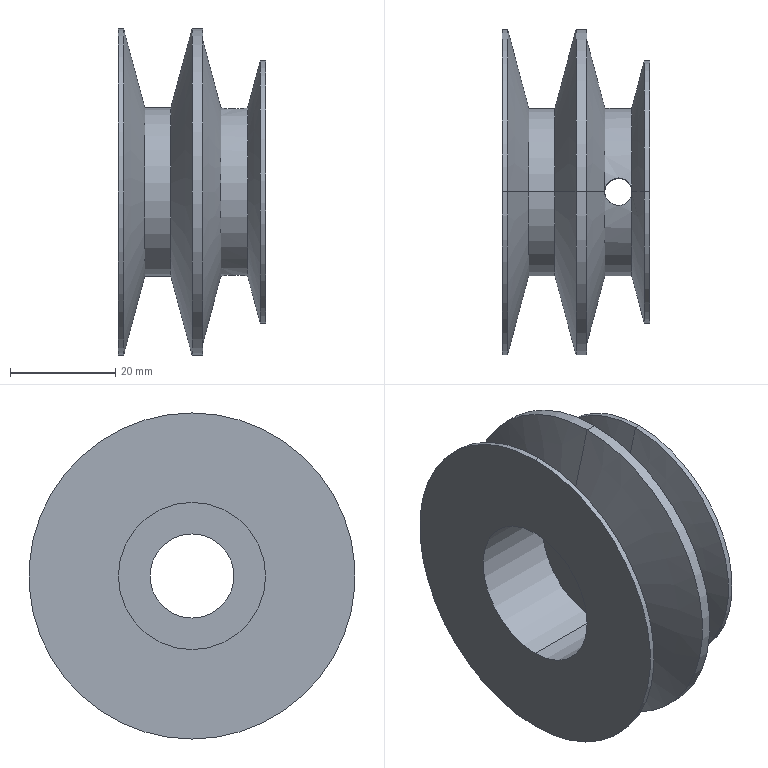Part | SolidWorks | features ICE 2, 3DProfileFeature 1, HoleWzd 1, Revolution 1 | 1 solid | 32 faces | box 28 x 62 x 62 mm | volume 29856 mm3 | cylinder 18 | cone 8 | plane 6 | commonest cylinder face diameters 5.22 x4 32 x4 62 x4 16 x2 28 x2 50 x2
STEP:
#1=CARTESIAN_POINT('',(-21.548,2.63,7.555));
#2=VERTEX_POINT('',#1);
#3=CARTESIAN_POINT('',(-24.158,0.,8.));
#4=VERTEX_POINT('',#3);
#5=CARTESIAN_POINT('',(-21.548,2.63,7.555));
#6=CARTESIAN_POINT('',(-21.72,2.63,7.555));
#7=CARTESIAN_POINT('',(-21.893,2.613,7.561));
#8=CARTESIAN_POINT('',(-22.233,2.545,7.585));
#9=CARTESIAN_POINT('',(-22.397,2.494,7.602));
#10=CARTESIAN_POINT('',(-22.713,2.362,7.644));
#11=CARTESIAN_POINT('',(-22.866,2.279,7.669));
#12=CARTESIAN_POINT('',(-23.149,2.089,7.723));
#13=CARTESIAN_POINT('',(-23.28,1.981,7.752));
#14=CARTESIAN_POINT('',(-23.642,1.616,7.839));
#15=CARTESIAN_POINT('',(-23.833,1.329,7.895));
#16=CARTESIAN_POINT('',(-24.029,0.8493,7.956));
#17=CARTESIAN_POINT('',(-24.078,0.6851,7.972));
#18=CARTESIAN_POINT('',(-24.143,0.3479,7.994));
#19=CARTESIAN_POINT('',(-24.159,0.1727,8.));
#20=CARTESIAN_POINT('',(-24.158,0.,8.));
#21=B_SPLINE_CURVE_WITH_KNOTS('',3,(#5,#6,#7,#8,#9,#10,#11,#12,#13,#14,#15,#16,#17,#18,#19,#20),.UNSPECIFIED.,.F.,.F.,(4,2,2,2,2,2,2,4),(0.008216,0.008732,0.009248,0.009764,0.01028,0.01131,0.01183,0.01234),.UNSPECIFIED.);
#22=EDGE_CURVE('',#2,#4,#21,.T.);
#23=ORIENTED_EDGE('',*,*,#22,.F.);
#24=CARTESIAN_POINT('',(-21.548,2.652,15.779));
#25=VERTEX_POINT('',#24);
#26=CARTESIAN_POINT('',(-21.548,2.653,15.993));
#27=DIRECTION('',(0.,0.002678,1.));
#28=VECTOR('',#27,1000.);
#29=LINE('',#26,#28);
#30=EDGE_CURVE('',#2,#25,#29,.T.);
#31=ORIENTED_EDGE('',*,*,#30,.T.);
#32=CARTESIAN_POINT('',(-24.127,0.4433,15.994));
#33=VERTEX_POINT('',#32);
#34=CARTESIAN_POINT('',(-24.127,0.4433,15.994));
#35=CARTESIAN_POINT('',(-24.079,0.7512,15.985));
#36=CARTESIAN_POINT('',(-23.979,1.043,15.968));
#37=CARTESIAN_POINT('',(-23.752,1.449,15.935));
#38=CARTESIAN_POINT('',(-23.666,1.576,15.923));
#39=CARTESIAN_POINT('',(-23.472,1.813,15.897));
#40=CARTESIAN_POINT('',(-23.363,1.924,15.884));
#41=CARTESIAN_POINT('',(-23.129,2.125,15.859));
#42=CARTESIAN_POINT('',(-23.004,2.214,15.846));
#43=CARTESIAN_POINT('',(-22.74,2.369,15.824));
#44=CARTESIAN_POINT('',(-22.599,2.436,15.814));
#45=CARTESIAN_POINT('',(-22.309,2.543,15.797));
#46=CARTESIAN_POINT('',(-22.161,2.584,15.79));
#47=CARTESIAN_POINT('',(-21.859,2.638,15.781));
#48=CARTESIAN_POINT('',(-21.702,2.652,15.779));
#49=CARTESIAN_POINT('',(-21.548,2.652,15.779));
#50=B_SPLINE_CURVE_WITH_KNOTS('',3,(#34,#35,#36,#37,#38,#39,#40,#41,#42,#43,#44,#45,#46,#47,#48,#49),.UNSPECIFIED.,.F.,.F.,(4,2,2,2,2,2,2,4),(0.,0.0009215,0.001382,0.001843,0.002304,0.002764,0.003225,0.003686),.UNSPECIFIED.);
#51=EDGE_CURVE('',#33,#25,#50,.T.);
#52=ORIENTED_EDGE('',*,*,#51,.F.);
#53=CARTESIAN_POINT('',(-24.128,0.435,15.999));
#54=VERTEX_POINT('',#53);
#55=CARTESIAN_POINT('',(-24.128,0.435,15.999));
#56=CARTESIAN_POINT('',(-24.128,0.4378,15.997));
#57=CARTESIAN_POINT('',(-24.127,0.4406,15.996));
#58=CARTESIAN_POINT('',(-24.127,0.4433,15.994));
#59=B_SPLINE_CURVE_WITH_KNOTS('',3,(#55,#56,#57,#58),.UNSPECIFIED.,.F.,.F.,(4,4),(0.0008614,0.0008711),.UNSPECIFIED.);
#60=EDGE_CURVE('',#54,#33,#59,.T.);
#61=ORIENTED_EDGE('',*,*,#60,.F.);
#62=CARTESIAN_POINT('',(-24.128,-0.3493,16.001));
#63=VERTEX_POINT('',#62);
#64=CARTESIAN_POINT('',(-21.548,0.04285,16.));
#65=DIRECTION('',(0.,0.002678,1.));
#66=DIRECTION('',(0.,-1.,0.002678));
#67=AXIS2_PLACEMENT_3D('',#64,#65,#66);
#68=CIRCLE('',#67,2.61);
#69=EDGE_CURVE('',#54,#63,#68,.T.);
#70=ORIENTED_EDGE('',*,*,#69,.T.);
#71=CARTESIAN_POINT('',(-24.127,-0.3577,15.996));
#72=VERTEX_POINT('',#71);
#73=CARTESIAN_POINT('',(-24.127,-0.3577,15.996));
#74=CARTESIAN_POINT('',(-24.127,-0.3549,15.998));
#75=CARTESIAN_POINT('',(-24.128,-0.3521,15.999));
#76=CARTESIAN_POINT('',(-24.128,-0.3493,16.001));
#77=B_SPLINE_CURVE_WITH_KNOTS('',3,(#73,#74,#75,#76),.UNSPECIFIED.,.F.,.F.,(4,4),(0.00002434,0.00003413),.UNSPECIFIED.);
#78=EDGE_CURVE('',#72,#63,#77,.T.);
#79=ORIENTED_EDGE('',*,*,#78,.F.);
#80=CARTESIAN_POINT('',(-21.548,-2.568,15.793));
#81=VERTEX_POINT('',#80);
#82=CARTESIAN_POINT('',(-21.548,-2.568,15.793));
#83=CARTESIAN_POINT('',(-21.703,-2.568,15.793));
#84=CARTESIAN_POINT('',(-21.858,-2.554,15.795));
#85=CARTESIAN_POINT('',(-22.16,-2.499,15.804));
#86=CARTESIAN_POINT('',(-22.309,-2.459,15.81));
#87=CARTESIAN_POINT('',(-22.746,-2.297,15.835));
#88=CARTESIAN_POINT('',(-23.011,-2.141,15.857));
#89=CARTESIAN_POINT('',(-23.364,-1.838,15.894));
#90=CARTESIAN_POINT('',(-23.471,-1.728,15.907));
#91=CARTESIAN_POINT('',(-23.665,-1.491,15.931));
#92=CARTESIAN_POINT('',(-23.752,-1.363,15.942));
#93=CARTESIAN_POINT('',(-23.978,-0.9574,15.974));
#94=CARTESIAN_POINT('',(-24.079,-0.6654,15.989));
#95=CARTESIAN_POINT('',(-24.127,-0.3577,15.996));
#96=B_SPLINE_CURVE_WITH_KNOTS('',3,(#82,#83,#84,#85,#86,#87,#88,#89,#90,#91,#92,#93,#94,#95),.UNSPECIFIED.,.F.,.F.,(4,2,2,2,2,2,4),(0.003428,0.003888,0.004349,0.00527,0.005731,0.006191,0.007113),.UNSPECIFIED.);
#97=EDGE_CURVE('',#81,#72,#96,.T.);
#98=ORIENTED_EDGE('',*,*,#97,.F.);
#99=CARTESIAN_POINT('',(-21.548,-2.59,7.569));
#100=VERTEX_POINT('',#99);
#101=CARTESIAN_POINT('',(-21.548,-2.567,16.007));
#102=DIRECTION('',(0.,0.002678,1.));
#103=VECTOR('',#102,1000.);
#104=LINE('',#101,#103);
#105=EDGE_CURVE('',#100,#81,#104,.T.);
#106=ORIENTED_EDGE('',*,*,#105,.F.);
#107=CARTESIAN_POINT('',(-24.158,0.,8.));
#108=CARTESIAN_POINT('',(-24.156,-0.1709,8.));
#109=CARTESIAN_POINT('',(-24.138,-0.3402,7.995));
#110=CARTESIAN_POINT('',(-24.069,-0.6754,7.973));
#111=CARTESIAN_POINT('',(-24.017,-0.8402,7.957));
#112=CARTESIAN_POINT('',(-23.819,-1.308,7.899));
#113=CARTESIAN_POINT('',(-23.625,-1.595,7.843));
#114=CARTESIAN_POINT('',(-23.267,-1.951,7.76));
#115=CARTESIAN_POINT('',(-23.134,-2.059,7.731));
#116=CARTESIAN_POINT('',(-22.852,-2.246,7.679));
#117=CARTESIAN_POINT('',(-22.704,-2.326,7.655));
#118=CARTESIAN_POINT('',(-22.39,-2.456,7.614));
#119=CARTESIAN_POINT('',(-22.224,-2.506,7.597));
#120=CARTESIAN_POINT('',(-21.891,-2.573,7.575));
#121=CARTESIAN_POINT('',(-21.721,-2.59,7.569));
#122=CARTESIAN_POINT('',(-21.548,-2.59,7.569));
#123=B_SPLINE_CURVE_WITH_KNOTS('',3,(#107,#108,#109,#110,#111,#112,#113,#114,#115,#116,#117,#118,#119,#120,#121,#122),.UNSPECIFIED.,.F.,.F.,(4,2,2,2,2,2,2,4),(0.01234,0.01285,0.01337,0.01439,0.0149,0.01541,0.01592,0.01643),.UNSPECIFIED.);
#124=EDGE_CURVE('',#4,#100,#123,.T.);
#125=ORIENTED_EDGE('',*,*,#124,.F.);
#126=EDGE_LOOP('',(#23,#31,#52,#61,#70,#79,#98,#106,#125));
#127=FACE_OUTER_BOUND('',#126,.T.);
#128=CARTESIAN_POINT('',(-21.548,0.04285,16.));
#129=DIRECTION('',(0.,0.002678,1.));
#130=DIRECTION('',(0.,-1.,0.002678));
#131=AXIS2_PLACEMENT_3D('',#128,#129,#130);
#132=CYLINDRICAL_SURFACE('',#131,2.61);
#133=ADVANCED_FACE('',(#127),#132,.F.);
#134=CARTESIAN_POINT('',(-21.548,2.568,-15.793));
#135=VERTEX_POINT('',#134);
#136=CARTESIAN_POINT('',(-24.127,0.3577,-15.996));
#137=VERTEX_POINT('',#136);
#138=CARTESIAN_POINT('',(-21.548,2.568,-15.793));
#139=CARTESIAN_POINT('',(-21.703,2.568,-15.793));
#140=CARTESIAN_POINT('',(-21.858,2.554,-15.795));
#141=CARTESIAN_POINT('',(-22.16,2.499,-15.804));
#142=CARTESIAN_POINT('',(-22.309,2.459,-15.81));
#143=CARTESIAN_POINT('',(-22.746,2.297,-15.835));
#144=CARTESIAN_POINT('',(-23.011,2.141,-15.857));
#145=CARTESIAN_POINT('',(-23.364,1.838,-15.894));
#146=CARTESIAN_POINT('',(-23.471,1.728,-15.907));
#147=CARTESIAN_POINT('',(-23.665,1.491,-15.931));
#148=CARTESIAN_POINT('',(-23.752,1.363,-15.942));
#149=CARTESIAN_POINT('',(-23.978,0.9574,-15.974));
#150=CARTESIAN_POINT('',(-24.079,0.6654,-15.989));
#151=CARTESIAN_POINT('',(-24.127,0.3577,-15.996));
#152=B_SPLINE_CURVE_WITH_KNOTS('',3,(#138,#139,#140,#141,#142,#143,#144,#145,#146,#147,#148,#149,#150,#151),.UNSPECIFIED.,.F.,.F.,(4,2,2,2,2,2,4),(0.003428,0.003888,0.004349,0.00527,0.005731,0.006191,0.007113),.UNSPECIFIED.);
#153=EDGE_CURVE('',#135,#137,#152,.T.);
#154=ORIENTED_EDGE('',*,*,#153,.F.);
#155=CARTESIAN_POINT('',(-21.548,2.59,-7.569));
#156=VERTEX_POINT('',#155);
#157=CARTESIAN_POINT('',(-21.548,2.653,15.993));
#158=DIRECTION('',(0.,0.002678,1.));
#159=VECTOR('',#158,1000.);
#160=LINE('',#157,#159);
#161=EDGE_CURVE('',#135,#156,#160,.T.);
#162=ORIENTED_EDGE('',*,*,#161,.T.);
#163=CARTESIAN_POINT('',(-24.158,0.,-8.));
#164=VERTEX_POINT('',#163);
#165=CARTESIAN_POINT('',(-24.158,0.,-8.));
#166=CARTESIAN_POINT('',(-24.156,0.1729,-8.));
#167=CARTESIAN_POINT('',(-24.138,0.3425,-7.994));
#168=CARTESIAN_POINT('',(-24.069,0.6756,-7.973));
#169=CARTESIAN_POINT('',(-24.017,0.8408,-7.957));
#170=CARTESIAN_POINT('',(-23.884,1.154,-7.918));
#171=CARTESIAN_POINT('',(-23.804,1.303,-7.895));
#172=CARTESIAN_POINT('',(-23.614,1.583,-7.843));
#173=CARTESIAN_POINT('',(-23.504,1.715,-7.815));
#174=CARTESIAN_POINT('',(-23.146,2.07,-7.731));
#175=CARTESIAN_POINT('',(-22.857,2.262,-7.675));
#176=CARTESIAN_POINT('',(-22.389,2.456,-7.614));
#177=CARTESIAN_POINT('',(-22.224,2.506,-7.597));
#178=CARTESIAN_POINT('',(-21.888,2.573,-7.575));
#179=CARTESIAN_POINT('',(-21.719,2.59,-7.569));
#180=CARTESIAN_POINT('',(-21.548,2.59,-7.569));
#181=B_SPLINE_CURVE_WITH_KNOTS('',3,(#165,#166,#167,#168,#169,#170,#171,#172,#173,#174,#175,#176,#177,#178,#179,#180),.UNSPECIFIED.,.F.,.F.,(4,2,2,2,2,2,2,4),(0.,0.000511,0.001022,0.001533,0.002044,0.003066,0.003577,0.004088),.UNSPECIFIED.);
#182=EDGE_CURVE('',#164,#156,#181,.T.);
#183=ORIENTED_EDGE('',*,*,#182,.F.);
#184=CARTESIAN_POINT('',(-21.548,-2.63,-7.555));
#185=VERTEX_POINT('',#184);
#186=CARTESIAN_POINT('',(-21.548,-2.63,-7.555));
#187=CARTESIAN_POINT('',(-21.721,-2.63,-7.555));
#188=CARTESIAN_POINT('',(-21.892,-2.613,-7.561));
#189=CARTESIAN_POINT('',(-22.231,-2.545,-7.584));
#190=CARTESIAN_POINT('',(-22.398,-2.494,-7.602));
#191=CARTESIAN_POINT('',(-22.871,-2.296,-7.665));
#192=CARTESIAN_POINT('',(-23.161,-2.1,-7.723));
#193=CARTESIAN_POINT('',(-23.52,-1.739,-7.81));
#194=CARTESIAN_POINT('',(-23.63,-1.604,-7.839));
#195=CARTESIAN_POINT('',(-23.818,-1.32,-7.892));
#196=CARTESIAN_POINT('',(-23.898,-1.169,-7.916));
#197=CARTESIAN_POINT('',(-24.028,-0.8517,-7.956));
#198=CARTESIAN_POINT('',(-24.078,-0.6839,-7.973));
#199=CARTESIAN_POINT('',(-24.143,-0.3463,-7.994));
#200=CARTESIAN_POINT('',(-24.159,-0.1746,-8.));
#201=CARTESIAN_POINT('',(-24.158,0.,-8.));
#202=B_SPLINE_CURVE_WITH_KNOTS('',3,(#186,#187,#188,#189,#190,#191,#192,#193,#194,#195,#196,#197,#198,#199,#200,#201),.UNSPECIFIED.,.F.,.F.,(4,2,2,2,2,2,2,4),(0.0123,0.01282,0.01333,0.01437,0.01488,0.0154,0.01591,0.01643),.UNSPECIFIED.);
#203=EDGE_CURVE('',#185,#164,#202,.T.);
#204=ORIENTED_EDGE('',*,*,#203,.F.);
#205=CARTESIAN_POINT('',(-21.548,-2.652,-15.779));
#206=VERTEX_POINT('',#205);
#207=CARTESIAN_POINT('',(-21.548,-2.567,16.007));
#208=DIRECTION('',(0.,0.002678,1.));
#209=VECTOR('',#208,1000.);
#210=LINE('',#207,#209);
#211=EDGE_CURVE('',#206,#185,#210,.T.);
#212=ORIENTED_EDGE('',*,*,#211,.F.);
#213=CARTESIAN_POINT('',(-24.127,-0.4433,-15.994));
#214=VERTEX_POINT('',#213);
#215=CARTESIAN_POINT('',(-24.127,-0.4433,-15.994));
#216=CARTESIAN_POINT('',(-24.079,-0.7512,-15.985));
#217=CARTESIAN_POINT('',(-23.979,-1.043,-15.968));
#218=CARTESIAN_POINT('',(-23.752,-1.449,-15.935));
#219=CARTESIAN_POINT('',(-23.666,-1.576,-15.923));
#220=CARTESIAN_POINT('',(-23.472,-1.813,-15.897));
#221=CARTESIAN_POINT('',(-23.363,-1.924,-15.884));
#222=CARTESIAN_POINT('',(-23.129,-2.125,-15.859));
#223=CARTESIAN_POINT('',(-23.004,-2.214,-15.846));
#224=CARTESIAN_POINT('',(-22.74,-2.369,-15.824));
#225=CARTESIAN_POINT('',(-22.599,-2.436,-15.814));
#226=CARTESIAN_POINT('',(-22.309,-2.543,-15.797));
#227=CARTESIAN_POINT('',(-22.161,-2.584,-15.79));
#228=CARTESIAN_POINT('',(-21.859,-2.638,-15.781));
#229=CARTESIAN_POINT('',(-21.702,-2.652,-15.779));
#230=CARTESIAN_POINT('',(-21.548,-2.652,-15.779));
#231=B_SPLINE_CURVE_WITH_KNOTS('',3,(#215,#216,#217,#218,#219,#220,#221,#222,#223,#224,#225,#226,#227,#228,#229,#230),.UNSPECIFIED.,.F.,.F.,(4,2,2,2,2,2,2,4),(0.,0.0009215,0.001382,0.001843,0.002304,0.002764,0.003225,0.003686),.UNSPECIFIED.);
#232=EDGE_CURVE('',#214,#206,#231,.T.);
#233=ORIENTED_EDGE('',*,*,#232,.F.);
#234=CARTESIAN_POINT('',(-24.158,0.,-16.114));
#235=VERTEX_POINT('',#234);
#236=CARTESIAN_POINT('',(-24.158,0.,-16.114));
#237=CARTESIAN_POINT('',(-24.159,-0.07704,-16.119));
#238=CARTESIAN_POINT('',(-24.157,-0.1564,-16.11));
#239=CARTESIAN_POINT('',(-24.146,-0.3055,-16.067));
#240=CARTESIAN_POINT('',(-24.137,-0.377,-16.034));
#241=CARTESIAN_POINT('',(-24.127,-0.4433,-15.994));
#242=B_SPLINE_CURVE_WITH_KNOTS('',3,(#236,#237,#238,#239,#240,#241),.UNSPECIFIED.,.F.,.F.,(4,2,4),(0.0004054,0.0006383,0.0008711),.UNSPECIFIED.);
#243=EDGE_CURVE('',#235,#214,#242,.T.);
#244=ORIENTED_EDGE('',*,*,#243,.F.);
#245=CARTESIAN_POINT('',(-24.127,0.3577,-15.996));
#246=CARTESIAN_POINT('',(-24.144,0.249,-16.061));
#247=CARTESIAN_POINT('',(-24.155,0.1261,-16.106));
#248=CARTESIAN_POINT('',(-24.158,0.,-16.114));
#249=B_SPLINE_CURVE_WITH_KNOTS('',3,(#245,#246,#247,#248),.UNSPECIFIED.,.F.,.F.,(4,4),(0.00002434,0.0004054),.UNSPECIFIED.);
#250=EDGE_CURVE('',#137,#235,#249,.T.);
#251=ORIENTED_EDGE('',*,*,#250,.F.);
#252=EDGE_LOOP('',(#154,#162,#183,#204,#212,#233,#244,#251));
#253=FACE_OUTER_BOUND('',#252,.T.);
#254=CARTESIAN_POINT('',(-21.548,0.04285,16.));
#255=DIRECTION('',(0.,0.002678,1.));
#256=DIRECTION('',(0.,-1.,0.002678));
#257=AXIS2_PLACEMENT_3D('',#254,#255,#256);
#258=CYLINDRICAL_SURFACE('',#257,2.61);
#259=ADVANCED_FACE('',(#253),#258,.F.);
#260=CARTESIAN_POINT('',(-27.61,0.,14.));
#261=VERTEX_POINT('',#260);
#262=CARTESIAN_POINT('',(-27.61,0.,-14.));
#263=VERTEX_POINT('',#262);
#264=CARTESIAN_POINT('',(-27.61,0.,0.));
#265=DIRECTION('',(1.,0.,0.));
#266=DIRECTION('',(0.,0.,1.));
#267=AXIS2_PLACEMENT_3D('',#264,#265,#266);
#268=CIRCLE('',#267,14.);
#269=EDGE_CURVE('',#261,#263,#268,.T.);
#270=ORIENTED_EDGE('',*,*,#269,.T.);
#271=CARTESIAN_POINT('',(-43.61,0.,-14.));
#272=VERTEX_POINT('',#271);
#273=CARTESIAN_POINT('',(11.988,0.,-14.));
#274=DIRECTION('',(-1.,0.,0.));
#275=VECTOR('',#274,1000.);
#276=LINE('',#273,#275);
#277=EDGE_CURVE('',#263,#272,#276,.T.);
#278=ORIENTED_EDGE('',*,*,#277,.T.);
#279=CARTESIAN_POINT('',(-43.61,0.,14.));
#280=VERTEX_POINT('',#279);
#281=CARTESIAN_POINT('',(-43.61,0.,0.));
#282=DIRECTION('',(-1.,0.,0.));
#283=DIRECTION('',(0.,0.,1.));
#284=AXIS2_PLACEMENT_3D('',#281,#282,#283);
#285=CIRCLE('',#284,14.);
#286=EDGE_CURVE('',#272,#280,#285,.T.);
#287=ORIENTED_EDGE('',*,*,#286,.T.);
#288=CARTESIAN_POINT('',(11.988,0.,14.));
#289=DIRECTION('',(-1.,0.,0.));
#290=VECTOR('',#289,1000.);
#291=LINE('',#288,#290);
#292=EDGE_CURVE('',#261,#280,#291,.T.);
#293=ORIENTED_EDGE('',*,*,#292,.F.);
#294=EDGE_LOOP('',(#270,#278,#287,#293));
#295=FACE_OUTER_BOUND('',#294,.T.);
#296=CARTESIAN_POINT('',(11.988,0.,0.));
#297=DIRECTION('',(-1.,0.,0.));
#298=DIRECTION('',(0.,0.,1.));
#299=AXIS2_PLACEMENT_3D('',#296,#297,#298);
#300=CYLINDRICAL_SURFACE('',#299,14.);
#301=ADVANCED_FACE('',(#295),#300,.F.);
#302=CARTESIAN_POINT('',(-15.61,0.,25.));
#303=VERTEX_POINT('',#302);
#304=CARTESIAN_POINT('',(-15.61,0.,-25.));
#305=VERTEX_POINT('',#304);
#306=CARTESIAN_POINT('',(-15.61,0.,0.));
#307=DIRECTION('',(-1.,0.,0.));
#308=DIRECTION('',(0.,0.,1.));
#309=AXIS2_PLACEMENT_3D('',#306,#307,#308);
#310=CIRCLE('',#309,25.);
#311=EDGE_CURVE('',#303,#305,#310,.T.);
#312=ORIENTED_EDGE('',*,*,#311,.T.);
#313=CARTESIAN_POINT('',(-16.61,0.,-25.));
#314=VERTEX_POINT('',#313);
#315=CARTESIAN_POINT('',(-65.147,0.,-25.));
#316=DIRECTION('',(-1.,0.,0.));
#317=VECTOR('',#316,1000.);
#318=LINE('',#315,#317);
#319=EDGE_CURVE('',#305,#314,#318,.T.);
#320=ORIENTED_EDGE('',*,*,#319,.T.);
#321=CARTESIAN_POINT('',(-16.61,0.,25.));
#322=VERTEX_POINT('',#321);
#323=CARTESIAN_POINT('',(-16.61,0.,0.));
#324=DIRECTION('',(-1.,0.,0.));
#325=DIRECTION('',(0.,0.,1.));
#326=AXIS2_PLACEMENT_3D('',#323,#324,#325);
#327=CIRCLE('',#326,25.);
#328=EDGE_CURVE('',#322,#314,#327,.T.);
#329=ORIENTED_EDGE('',*,*,#328,.F.);
#330=CARTESIAN_POINT('',(-65.147,0.,25.));
#331=DIRECTION('',(-1.,0.,0.));
#332=VECTOR('',#331,1000.);
#333=LINE('',#330,#332);
#334=EDGE_CURVE('',#303,#322,#333,.T.);
#335=ORIENTED_EDGE('',*,*,#334,.F.);
#336=EDGE_LOOP('',(#312,#320,#329,#335));
#337=FACE_OUTER_BOUND('',#336,.T.);
#338=CARTESIAN_POINT('',(-65.147,0.,0.));
#339=DIRECTION('',(-1.,0.,0.));
#340=DIRECTION('',(0.,0.,1.));
#341=AXIS2_PLACEMENT_3D('',#338,#339,#340);
#342=CYLINDRICAL_SURFACE('',#341,25.);
#343=ADVANCED_FACE('',(#337),#342,.T.);
#344=CARTESIAN_POINT('',(-19.018,0.6849,15.998));
#345=VERTEX_POINT('',#344);
#346=CARTESIAN_POINT('',(-19.022,0.,16.));
#347=VERTEX_POINT('',#346);
#348=CARTESIAN_POINT('',(-19.018,0.6849,15.998));
#349=CARTESIAN_POINT('',(-19.021,0.4566,15.999));
#350=CARTESIAN_POINT('',(-19.022,0.2283,15.999));
#351=CARTESIAN_POINT('',(-19.022,0.,16.));
#352=B_SPLINE_CURVE_WITH_KNOTS('',3,(#348,#349,#350,#351),.UNSPECIFIED.,.F.,.F.,(4,4),(0.001968,0.002653),.UNSPECIFIED.);
#353=EDGE_CURVE('',#345,#347,#352,.T.);
#354=ORIENTED_EDGE('',*,*,#353,.T.);
#355=CARTESIAN_POINT('',(-16.61,0.,25.));
#356=DIRECTION('',(0.2588,0.,0.9659));
#357=VECTOR('',#356,1000.);
#358=LINE('',#355,#357);
#359=EDGE_CURVE('',#347,#322,#358,.T.);
#360=ORIENTED_EDGE('',*,*,#359,.T.);
#361=ORIENTED_EDGE('',*,*,#328,.T.);
#362=CARTESIAN_POINT('',(-18.939,0.,-16.311));
#363=VERTEX_POINT('',#362);
#364=CARTESIAN_POINT('',(-16.61,0.,-25.));
#365=DIRECTION('',(0.2588,0.,-0.9659));
#366=VECTOR('',#365,1000.);
#367=LINE('',#364,#366);
#368=EDGE_CURVE('',#363,#314,#367,.T.);
#369=ORIENTED_EDGE('',*,*,#368,.F.);
#370=CARTESIAN_POINT('',(-19.022,0.6127,-15.988));
#371=VERTEX_POINT('',#370);
#372=CARTESIAN_POINT('',(-18.939,0.,-16.311));
#373=CARTESIAN_POINT('',(-18.941,0.1198,-16.303));
#374=CARTESIAN_POINT('',(-18.951,0.2345,-16.263));
#375=CARTESIAN_POINT('',(-18.981,0.4384,-16.147));
#376=CARTESIAN_POINT('',(-19.,0.53,-16.071));
#377=CARTESIAN_POINT('',(-19.022,0.6127,-15.988));
#378=B_SPLINE_CURVE_WITH_KNOTS('',3,(#372,#373,#374,#375,#376,#377),.UNSPECIFIED.,.F.,.F.,(4,2,4),(0.0008458,0.001201,0.001557),.UNSPECIFIED.);
#379=EDGE_CURVE('',#363,#371,#378,.T.);
#380=ORIENTED_EDGE('',*,*,#379,.T.);
#381=CARTESIAN_POINT('',(-19.022,0.6983,15.985));
#382=VERTEX_POINT('',#381);
#383=CARTESIAN_POINT('',(-19.022,0.,0.));
#384=DIRECTION('',(-1.,0.,0.));
#385=DIRECTION('',(0.,0.,1.));
#386=AXIS2_PLACEMENT_3D('',#383,#384,#385);
#387=CIRCLE('',#386,16.);
#388=EDGE_CURVE('',#382,#371,#387,.T.);
#389=ORIENTED_EDGE('',*,*,#388,.F.);
#390=CARTESIAN_POINT('',(-19.022,0.6983,15.985));
#391=CARTESIAN_POINT('',(-19.021,0.6939,15.989));
#392=CARTESIAN_POINT('',(-19.02,0.6894,15.994));
#393=CARTESIAN_POINT('',(-19.018,0.6849,15.998));
#394=B_SPLINE_CURVE_WITH_KNOTS('',3,(#390,#391,#392,#393),.UNSPECIFIED.,.F.,.F.,(4,4),(0.00004691,0.00006616),.UNSPECIFIED.);
#395=EDGE_CURVE('',#382,#345,#394,.T.);
#396=ORIENTED_EDGE('',*,*,#395,.T.);
#397=EDGE_LOOP('',(#354,#360,#361,#369,#380,#389,#396));
#398=FACE_OUTER_BOUND('',#397,.T.);
#399=CARTESIAN_POINT('',(-16.61,0.,0.));
#400=DIRECTION('',(1.,0.,0.));
#401=DIRECTION('',(0.,0.,-1.));
#402=AXIS2_PLACEMENT_3D('',#399,#400,#401);
#403=CONICAL_SURFACE('',#402,25.,1.309);
#404=ADVANCED_FACE('',(#398),#403,.T.);
#405=ORIENTED_EDGE('',*,*,#250,.T.);
#406=CARTESIAN_POINT('',(-27.61,0.,-29.));
#407=VERTEX_POINT('',#406);
#408=CARTESIAN_POINT('',(-24.127,0.,-16.));
#409=DIRECTION('',(-0.2588,0.,-0.9659));
#410=VECTOR('',#409,1000.);
#411=LINE('',#408,#410);
#412=EDGE_CURVE('',#235,#407,#411,.T.);
#413=ORIENTED_EDGE('',*,*,#412,.T.);
#414=CARTESIAN_POINT('',(-27.61,0.,29.));
#415=VERTEX_POINT('',#414);
#416=CARTESIAN_POINT('',(-27.61,0.,0.));
#417=DIRECTION('',(-1.,0.,0.));
#418=DIRECTION('',(0.,0.,1.));
#419=AXIS2_PLACEMENT_3D('',#416,#417,#418);
#420=CIRCLE('',#419,29.);
#421=EDGE_CURVE('',#415,#407,#420,.T.);
#422=ORIENTED_EDGE('',*,*,#421,.F.);
#423=CARTESIAN_POINT('',(-24.127,0.,16.));
#424=VERTEX_POINT('',#423);
#425=CARTESIAN_POINT('',(-24.127,0.,16.));
#426=DIRECTION('',(-0.2588,0.,0.9659));
#427=VECTOR('',#426,1000.);
#428=LINE('',#425,#427);
#429=EDGE_CURVE('',#424,#415,#428,.T.);
#430=ORIENTED_EDGE('',*,*,#429,.F.);
#431=CARTESIAN_POINT('',(-24.127,0.,16.));
#432=CARTESIAN_POINT('',(-24.127,0.145,16.));
#433=CARTESIAN_POINT('',(-24.127,0.29,15.999));
#434=CARTESIAN_POINT('',(-24.128,0.435,15.999));
#435=B_SPLINE_CURVE_WITH_KNOTS('',3,(#431,#432,#433,#434),.UNSPECIFIED.,.F.,.F.,(4,4),(0.001888,0.002323),.UNSPECIFIED.);
#436=EDGE_CURVE('',#424,#54,#435,.T.);
#437=ORIENTED_EDGE('',*,*,#436,.T.);
#438=ORIENTED_EDGE('',*,*,#60,.T.);
#439=CARTESIAN_POINT('',(-24.127,0.,0.));
#440=DIRECTION('',(-1.,0.,0.));
#441=DIRECTION('',(0.,0.,1.));
#442=AXIS2_PLACEMENT_3D('',#439,#440,#441);
#443=CIRCLE('',#442,16.);
#444=EDGE_CURVE('',#33,#137,#443,.T.);
#445=ORIENTED_EDGE('',*,*,#444,.T.);
#446=EDGE_LOOP('',(#405,#413,#422,#430,#437,#438,#445));
#447=FACE_OUTER_BOUND('',#446,.T.);
#448=CARTESIAN_POINT('',(-24.127,0.,0.));
#449=DIRECTION('',(-1.,0.,0.));
#450=DIRECTION('',(0.,0.,1.));
#451=AXIS2_PLACEMENT_3D('',#448,#449,#450);
#452=CONICAL_SURFACE('',#451,16.,1.309);
#453=ADVANCED_FACE('',(#447),#452,.T.);
#454=CARTESIAN_POINT('',(-27.61,0.,31.));
#455=VERTEX_POINT('',#454);
#456=CARTESIAN_POINT('',(-27.61,0.,-31.));
#457=VERTEX_POINT('',#456);
#458=CARTESIAN_POINT('',(-27.61,0.,0.));
#459=DIRECTION('',(-1.,0.,0.));
#460=DIRECTION('',(0.,0.,1.));
#461=AXIS2_PLACEMENT_3D('',#458,#459,#460);
#462=CIRCLE('',#461,31.);
#463=EDGE_CURVE('',#455,#457,#462,.T.);
#464=ORIENTED_EDGE('',*,*,#463,.T.);
#465=CARTESIAN_POINT('',(-29.61,0.,-31.));
#466=VERTEX_POINT('',#465);
#467=CARTESIAN_POINT('',(-65.147,0.,-31.));
#468=DIRECTION('',(-1.,0.,0.));
#469=VECTOR('',#468,1000.);
#470=LINE('',#467,#469);
#471=EDGE_CURVE('',#457,#466,#470,.T.);
#472=ORIENTED_EDGE('',*,*,#471,.T.);
#473=CARTESIAN_POINT('',(-29.61,0.,31.));
#474=VERTEX_POINT('',#473);
#475=CARTESIAN_POINT('',(-29.61,0.,0.));
#476=DIRECTION('',(-1.,0.,0.));
#477=DIRECTION('',(0.,0.,1.));
#478=AXIS2_PLACEMENT_3D('',#475,#476,#477);
#479=CIRCLE('',#478,31.);
#480=EDGE_CURVE('',#474,#466,#479,.T.);
#481=ORIENTED_EDGE('',*,*,#480,.F.);
#482=CARTESIAN_POINT('',(-65.147,0.,31.));
#483=DIRECTION('',(-1.,0.,0.));
#484=VECTOR('',#483,1000.);
#485=LINE('',#482,#484);
#486=EDGE_CURVE('',#455,#474,#485,.T.);
#487=ORIENTED_EDGE('',*,*,#486,.F.);
#488=EDGE_LOOP('',(#464,#472,#481,#487));
#489=FACE_OUTER_BOUND('',#488,.T.);
#490=CARTESIAN_POINT('',(-65.147,0.,0.));
#491=DIRECTION('',(-1.,0.,0.));
#492=DIRECTION('',(0.,0.,1.));
#493=AXIS2_PLACEMENT_3D('',#490,#491,#492);
#494=CYLINDRICAL_SURFACE('',#493,31.);
#495=ADVANCED_FACE('',(#489),#494,.T.);
#496=CARTESIAN_POINT('',(-33.63,0.,16.));
#497=VERTEX_POINT('',#496);
#498=CARTESIAN_POINT('',(-33.63,0.,-16.));
#499=VERTEX_POINT('',#498);
#500=CARTESIAN_POINT('',(-33.63,0.,0.));
#501=DIRECTION('',(-1.,0.,0.));
#502=DIRECTION('',(0.,0.,1.));
#503=AXIS2_PLACEMENT_3D('',#500,#501,#502);
#504=CIRCLE('',#503,16.);
#505=EDGE_CURVE('',#497,#499,#504,.T.);
#506=ORIENTED_EDGE('',*,*,#505,.F.);
#507=CARTESIAN_POINT('',(-29.61,0.,31.));
#508=DIRECTION('',(0.2588,0.,0.9659));
#509=VECTOR('',#508,1000.);
#510=LINE('',#507,#509);
#511=EDGE_CURVE('',#497,#474,#510,.T.);
#512=ORIENTED_EDGE('',*,*,#511,.T.);
#513=ORIENTED_EDGE('',*,*,#480,.T.);
#514=CARTESIAN_POINT('',(-29.61,0.,-31.));
#515=DIRECTION('',(0.2588,0.,-0.9659));
#516=VECTOR('',#515,1000.);
#517=LINE('',#514,#516);
#518=EDGE_CURVE('',#499,#466,#517,.T.);
#519=ORIENTED_EDGE('',*,*,#518,.F.);
#520=EDGE_LOOP('',(#506,#512,#513,#519));
#521=FACE_OUTER_BOUND('',#520,.T.);
#522=CARTESIAN_POINT('',(-29.61,0.,0.));
#523=DIRECTION('',(1.,0.,0.));
#524=DIRECTION('',(0.,0.,-1.));
#525=AXIS2_PLACEMENT_3D('',#522,#523,#524);
#526=CONICAL_SURFACE('',#525,31.,1.309);
#527=ADVANCED_FACE('',(#521),#526,.T.);
#528=ORIENTED_EDGE('',*,*,#505,.T.);
#529=CARTESIAN_POINT('',(-38.591,0.,-16.));
#530=VERTEX_POINT('',#529);
#531=CARTESIAN_POINT('',(-65.147,0.,-16.));
#532=DIRECTION('',(-1.,0.,0.));
#533=VECTOR('',#532,1000.);
#534=LINE('',#531,#533);
#535=EDGE_CURVE('',#499,#530,#534,.T.);
#536=ORIENTED_EDGE('',*,*,#535,.T.);
#537=CARTESIAN_POINT('',(-38.591,0.,16.));
#538=VERTEX_POINT('',#537);
#539=CARTESIAN_POINT('',(-38.591,0.,0.));
#540=DIRECTION('',(-1.,0.,0.));
#541=DIRECTION('',(0.,0.,1.));
#542=AXIS2_PLACEMENT_3D('',#539,#540,#541);
#543=CIRCLE('',#542,16.);
#544=EDGE_CURVE('',#538,#530,#543,.T.);
#545=ORIENTED_EDGE('',*,*,#544,.F.);
#546=CARTESIAN_POINT('',(-65.147,0.,16.));
#547=DIRECTION('',(-1.,0.,0.));
#548=VECTOR('',#547,1000.);
#549=LINE('',#546,#548);
#550=EDGE_CURVE('',#497,#538,#549,.T.);
#551=ORIENTED_EDGE('',*,*,#550,.F.);
#552=EDGE_LOOP('',(#528,#536,#545,#551));
#553=FACE_OUTER_BOUND('',#552,.T.);
#554=CARTESIAN_POINT('',(-65.147,0.,0.));
#555=DIRECTION('',(-1.,0.,0.));
#556=DIRECTION('',(0.,0.,1.));
#557=AXIS2_PLACEMENT_3D('',#554,#555,#556);
#558=CYLINDRICAL_SURFACE('',#557,16.);
#559=ADVANCED_FACE('',(#553),#558,.T.);
#560=ORIENTED_EDGE('',*,*,#544,.T.);
#561=CARTESIAN_POINT('',(-42.61,0.,-31.));
#562=VERTEX_POINT('',#561);
#563=CARTESIAN_POINT('',(-38.591,0.,-16.));
#564=DIRECTION('',(-0.2588,0.,-0.9659));
#565=VECTOR('',#564,1000.);
#566=LINE('',#563,#565);
#567=EDGE_CURVE('',#530,#562,#566,.T.);
#568=ORIENTED_EDGE('',*,*,#567,.T.);
#569=CARTESIAN_POINT('',(-42.61,0.,31.));
#570=VERTEX_POINT('',#569);
#571=CARTESIAN_POINT('',(-42.61,0.,0.));
#572=DIRECTION('',(-1.,0.,0.));
#573=DIRECTION('',(0.,0.,1.));
#574=AXIS2_PLACEMENT_3D('',#571,#572,#573);
#575=CIRCLE('',#574,31.);
#576=EDGE_CURVE('',#570,#562,#575,.T.);
#577=ORIENTED_EDGE('',*,*,#576,.F.);
#578=CARTESIAN_POINT('',(-38.591,0.,16.));
#579=DIRECTION('',(-0.2588,0.,0.9659));
#580=VECTOR('',#579,1000.);
#581=LINE('',#578,#580);
#582=EDGE_CURVE('',#538,#570,#581,.T.);
#583=ORIENTED_EDGE('',*,*,#582,.F.);
#584=EDGE_LOOP('',(#560,#568,#577,#583));
#585=FACE_OUTER_BOUND('',#584,.T.);
#586=CARTESIAN_POINT('',(-38.591,0.,0.));
#587=DIRECTION('',(-1.,0.,0.));
#588=DIRECTION('',(0.,0.,1.));
#589=AXIS2_PLACEMENT_3D('',#586,#587,#588);
#590=CONICAL_SURFACE('',#589,16.,1.309);
#591=ADVANCED_FACE('',(#585),#590,.T.);
#592=ORIENTED_EDGE('',*,*,#576,.T.);
#593=CARTESIAN_POINT('',(-43.61,0.,-31.));
#594=VERTEX_POINT('',#593);
#595=CARTESIAN_POINT('',(-65.147,0.,-31.));
#596=DIRECTION('',(-1.,0.,0.));
#597=VECTOR('',#596,1000.);
#598=LINE('',#595,#597);
#599=EDGE_CURVE('',#562,#594,#598,.T.);
#600=ORIENTED_EDGE('',*,*,#599,.T.);
#601=CARTESIAN_POINT('',(-43.61,0.,31.));
#602=VERTEX_POINT('',#601);
#603=CARTESIAN_POINT('',(-43.61,0.,0.));
#604=DIRECTION('',(-1.,0.,0.));
#605=DIRECTION('',(0.,0.,1.));
#606=AXIS2_PLACEMENT_3D('',#603,#604,#605);
#607=CIRCLE('',#606,31.);
#608=EDGE_CURVE('',#602,#594,#607,.T.);
#609=ORIENTED_EDGE('',*,*,#608,.F.);
#610=CARTESIAN_POINT('',(-65.147,0.,31.));
#611=DIRECTION('',(-1.,0.,0.));
#612=VECTOR('',#611,1000.);
#613=LINE('',#610,#612);
#614=EDGE_CURVE('',#570,#602,#613,.T.);
#615=ORIENTED_EDGE('',*,*,#614,.F.);
#616=EDGE_LOOP('',(#592,#600,#609,#615));
#617=FACE_OUTER_BOUND('',#616,.T.);
#618=CARTESIAN_POINT('',(-65.147,0.,0.));
#619=DIRECTION('',(-1.,0.,0.));
#620=DIRECTION('',(0.,0.,1.));
#621=AXIS2_PLACEMENT_3D('',#618,#619,#620);
#622=CYLINDRICAL_SURFACE('',#621,31.);
#623=ADVANCED_FACE('',(#617),#622,.T.);
#624=CARTESIAN_POINT('',(-27.61,0.,8.));
#625=VERTEX_POINT('',#624);
#626=CARTESIAN_POINT('',(-27.61,0.,-8.));
#627=VERTEX_POINT('',#626);
#628=CARTESIAN_POINT('',(-27.61,0.,0.));
#629=DIRECTION('',(1.,0.,0.));
#630=DIRECTION('',(0.,0.,1.));
#631=AXIS2_PLACEMENT_3D('',#628,#629,#630);
#632=CIRCLE('',#631,8.);
#633=EDGE_CURVE('',#625,#627,#632,.T.);
#634=ORIENTED_EDGE('',*,*,#633,.F.);
#635=CARTESIAN_POINT('',(-43.61,0.,8.));
#636=DIRECTION('',(1.,0.,0.));
#637=VECTOR('',#636,1000.);
#638=LINE('',#635,#637);
#639=EDGE_CURVE('',#625,#4,#638,.T.);
#640=ORIENTED_EDGE('',*,*,#639,.T.);
#641=ORIENTED_EDGE('',*,*,#124,.T.);
#642=CARTESIAN_POINT('',(-18.938,0.,8.));
#643=VERTEX_POINT('',#642);
#644=CARTESIAN_POINT('',(-21.548,-2.59,7.569));
#645=CARTESIAN_POINT('',(-21.375,-2.59,7.569));
#646=CARTESIAN_POINT('',(-21.205,-2.573,7.575));
#647=CARTESIAN_POINT('',(-20.872,-2.506,7.597));
#648=CARTESIAN_POINT('',(-20.706,-2.456,7.614));
#649=CARTESIAN_POINT('',(-20.392,-2.326,7.655));
#650=CARTESIAN_POINT('',(-20.243,-2.246,7.679));
#651=CARTESIAN_POINT('',(-19.961,-2.058,7.731));
#652=CARTESIAN_POINT('',(-19.829,-1.95,7.76));
#653=CARTESIAN_POINT('',(-19.471,-1.594,7.843));
#654=CARTESIAN_POINT('',(-19.276,-1.307,7.899));
#655=CARTESIAN_POINT('',(-19.079,-0.84,7.957));
#656=CARTESIAN_POINT('',(-19.027,-0.6756,7.973));
#657=CARTESIAN_POINT('',(-18.958,-0.3399,7.995));
#658=CARTESIAN_POINT('',(-18.94,-0.1706,8.));
#659=CARTESIAN_POINT('',(-18.938,0.,8.));
#660=B_SPLINE_CURVE_WITH_KNOTS('',3,(#644,#645,#646,#647,#648,#649,#650,#651,#652,#653,#654,#655,#656,#657,#658,#659),.UNSPECIFIED.,.F.,.F.,(4,2,2,2,2,2,2,4),(0.,0.000511,0.001022,0.001533,0.002044,0.003066,0.003577,0.004088),.UNSPECIFIED.);
#661=EDGE_CURVE('',#100,#643,#660,.T.);
#662=ORIENTED_EDGE('',*,*,#661,.T.);
#663=CARTESIAN_POINT('',(-15.61,0.,8.));
#664=VERTEX_POINT('',#663);
#665=CARTESIAN_POINT('',(-43.61,0.,8.));
#666=DIRECTION('',(1.,0.,0.));
#667=VECTOR('',#666,1000.);
#668=LINE('',#665,#667);
#669=EDGE_CURVE('',#643,#664,#668,.T.);
#670=ORIENTED_EDGE('',*,*,#669,.T.);
#671=CARTESIAN_POINT('',(-15.61,0.,-8.));
#672=VERTEX_POINT('',#671);
#673=CARTESIAN_POINT('',(-15.61,0.,0.));
#674=DIRECTION('',(1.,0.,0.));
#675=DIRECTION('',(0.,0.,-1.));
#676=AXIS2_PLACEMENT_3D('',#673,#674,#675);
#677=CIRCLE('',#676,8.);
#678=EDGE_CURVE('',#664,#672,#677,.T.);
#679=ORIENTED_EDGE('',*,*,#678,.T.);
#680=CARTESIAN_POINT('',(-18.938,0.,-8.));
#681=VERTEX_POINT('',#680);
#682=CARTESIAN_POINT('',(-43.61,0.,-8.));
#683=DIRECTION('',(1.,0.,0.));
#684=VECTOR('',#683,1000.);
#685=LINE('',#682,#684);
#686=EDGE_CURVE('',#681,#672,#685,.T.);
#687=ORIENTED_EDGE('',*,*,#686,.F.);
#688=CARTESIAN_POINT('',(-18.938,0.,-8.));
#689=CARTESIAN_POINT('',(-18.935,-0.3441,-8.));
#690=CARTESIAN_POINT('',(-19.003,-0.6919,-7.976));
#691=CARTESIAN_POINT('',(-19.197,-1.167,-7.916));
#692=CARTESIAN_POINT('',(-19.279,-1.321,-7.891));
#693=CARTESIAN_POINT('',(-19.467,-1.606,-7.839));
#694=CARTESIAN_POINT('',(-19.575,-1.737,-7.81));
#695=CARTESIAN_POINT('',(-19.816,-1.98,-7.752));
#696=CARTESIAN_POINT('',(-19.949,-2.09,-7.723));
#697=CARTESIAN_POINT('',(-20.23,-2.28,-7.669));
#698=CARTESIAN_POINT('',(-20.381,-2.361,-7.644));
#699=CARTESIAN_POINT('',(-20.7,-2.495,-7.601));
#700=CARTESIAN_POINT('',(-20.864,-2.545,-7.585));
#701=CARTESIAN_POINT('',(-21.2,-2.613,-7.561));
#702=CARTESIAN_POINT('',(-21.375,-2.63,-7.555));
#703=CARTESIAN_POINT('',(-21.548,-2.63,-7.555));
#704=B_SPLINE_CURVE_WITH_KNOTS('',3,(#688,#689,#690,#691,#692,#693,#694,#695,#696,#697,#698,#699,#700,#701,#702,#703),.UNSPECIFIED.,.F.,.F.,(4,2,2,2,2,2,2,4),(0.008173,0.009205,0.009721,0.01024,0.01075,0.01127,0.01179,0.0123),.UNSPECIFIED.);
#705=EDGE_CURVE('',#681,#185,#704,.T.);
#706=ORIENTED_EDGE('',*,*,#705,.T.);
#707=ORIENTED_EDGE('',*,*,#203,.T.);
#708=CARTESIAN_POINT('',(-43.61,0.,-8.));
#709=DIRECTION('',(1.,0.,0.));
#710=VECTOR('',#709,1000.);
#711=LINE('',#708,#710);
#712=EDGE_CURVE('',#627,#164,#711,.T.);
#713=ORIENTED_EDGE('',*,*,#712,.F.);
#714=EDGE_LOOP('',(#634,#640,#641,#662,#670,#679,#687,#706,#707,#713));
#715=FACE_OUTER_BOUND('',#714,.T.);
#716=CARTESIAN_POINT('',(-43.61,0.,0.));
#717=DIRECTION('',(1.,0.,0.));
#718=DIRECTION('',(0.,0.,-1.));
#719=AXIS2_PLACEMENT_3D('',#716,#717,#718);
#720=CYLINDRICAL_SURFACE('',#719,8.);
#721=ADVANCED_FACE('',(#715),#720,.F.);
#722=ORIENTED_EDGE('',*,*,#388,.T.);
#723=CARTESIAN_POINT('',(-19.022,0.6127,-15.988));
#724=CARTESIAN_POINT('',(-19.095,0.893,-15.978));
#725=CARTESIAN_POINT('',(-19.211,1.154,-15.96));
#726=CARTESIAN_POINT('',(-19.528,1.635,-15.918));
#727=CARTESIAN_POINT('',(-19.723,1.845,-15.894));
#728=CARTESIAN_POINT('',(-20.178,2.198,-15.849));
#729=CARTESIAN_POINT('',(-20.43,2.334,-15.829));
#730=CARTESIAN_POINT('',(-20.976,2.52,-15.801));
#731=CARTESIAN_POINT('',(-21.26,2.568,-15.793));
#732=CARTESIAN_POINT('',(-21.548,2.568,-15.793));
#733=B_SPLINE_CURVE_WITH_KNOTS('',3,(#723,#724,#725,#726,#727,#728,#729,#730,#731,#732),.UNSPECIFIED.,.F.,.F.,(4,2,2,2,4),(0.,0.000857,0.001714,0.002571,0.003428),.UNSPECIFIED.);
#734=EDGE_CURVE('',#371,#135,#733,.T.);
#735=ORIENTED_EDGE('',*,*,#734,.T.);
#736=ORIENTED_EDGE('',*,*,#153,.T.);
#737=ORIENTED_EDGE('',*,*,#444,.F.);
#738=ORIENTED_EDGE('',*,*,#51,.T.);
#739=CARTESIAN_POINT('',(-21.548,2.652,15.779));
#740=CARTESIAN_POINT('',(-21.405,2.652,15.779));
#741=CARTESIAN_POINT('',(-21.262,2.64,15.781));
#742=CARTESIAN_POINT('',(-20.98,2.594,15.788));
#743=CARTESIAN_POINT('',(-20.839,2.558,15.794));
#744=CARTESIAN_POINT('',(-20.567,2.465,15.809));
#745=CARTESIAN_POINT('',(-20.437,2.408,15.818));
#746=CARTESIAN_POINT('',(-20.185,2.273,15.838));
#747=CARTESIAN_POINT('',(-20.064,2.194,15.849));
#748=CARTESIAN_POINT('',(-19.837,2.019,15.872));
#749=CARTESIAN_POINT('',(-19.732,1.922,15.884));
#750=CARTESIAN_POINT('',(-19.538,1.714,15.908));
#751=CARTESIAN_POINT('',(-19.449,1.6,15.92));
#752=CARTESIAN_POINT('',(-19.212,1.241,15.954));
#753=CARTESIAN_POINT('',(-19.095,0.9785,15.973));
#754=CARTESIAN_POINT('',(-19.022,0.6983,15.985));
#755=B_SPLINE_CURVE_WITH_KNOTS('',3,(#739,#740,#741,#742,#743,#744,#745,#746,#747,#748,#749,#750,#751,#752,#753,#754),.UNSPECIFIED.,.F.,.F.,(4,2,2,2,2,2,2,4),(0.003686,0.004114,0.004543,0.004971,0.005399,0.005828,0.006256,0.007113),.UNSPECIFIED.);
#756=EDGE_CURVE('',#25,#382,#755,.T.);
#757=ORIENTED_EDGE('',*,*,#756,.T.);
#758=EDGE_LOOP('',(#722,#735,#736,#737,#738,#757));
#759=FACE_OUTER_BOUND('',#758,.T.);
#760=CARTESIAN_POINT('',(-65.147,0.,0.));
#761=DIRECTION('',(-1.,0.,0.));
#762=DIRECTION('',(0.,0.,1.));
#763=AXIS2_PLACEMENT_3D('',#760,#761,#762);
#764=CYLINDRICAL_SURFACE('',#763,16.);
#765=ADVANCED_FACE('',(#759),#764,.T.);
#766=ORIENTED_EDGE('',*,*,#639,.F.);
#767=CARTESIAN_POINT('',(-27.61,0.,0.));
#768=DIRECTION('',(1.,0.,0.));
#769=DIRECTION('',(0.,0.,1.));
#770=AXIS2_PLACEMENT_3D('',#767,#768,#769);
#771=CIRCLE('',#770,8.);
#772=EDGE_CURVE('',#627,#625,#771,.T.);
#773=ORIENTED_EDGE('',*,*,#772,.F.);
#774=ORIENTED_EDGE('',*,*,#712,.T.);
#775=ORIENTED_EDGE('',*,*,#182,.T.);
#776=CARTESIAN_POINT('',(-21.548,2.59,-7.569));
#777=CARTESIAN_POINT('',(-21.378,2.59,-7.569));
#778=CARTESIAN_POINT('',(-21.204,2.572,-7.575));
#779=CARTESIAN_POINT('',(-20.87,2.506,-7.598));
#780=CARTESIAN_POINT('',(-20.708,2.456,-7.614));
#781=CARTESIAN_POINT('',(-20.234,2.26,-7.675));
#782=CARTESIAN_POINT('',(-19.949,2.07,-7.732));
#783=CARTESIAN_POINT('',(-19.589,1.712,-7.816));
#784=CARTESIAN_POINT('',(-19.482,1.582,-7.843));
#785=CARTESIAN_POINT('',(-19.293,1.303,-7.894));
#786=CARTESIAN_POINT('',(-19.21,1.151,-7.918));
#787=CARTESIAN_POINT('',(-19.078,0.8391,-7.957));
#788=CARTESIAN_POINT('',(-19.028,0.6775,-7.973));
#789=CARTESIAN_POINT('',(-18.958,0.3428,-7.994));
#790=CARTESIAN_POINT('',(-18.94,0.1702,-8.));
#791=CARTESIAN_POINT('',(-18.938,0.,-8.));
#792=B_SPLINE_CURVE_WITH_KNOTS('',3,(#776,#777,#778,#779,#780,#781,#782,#783,#784,#785,#786,#787,#788,#789,#790,#791),.UNSPECIFIED.,.F.,.F.,(4,2,2,2,2,2,2,4),(0.004088,0.004599,0.005109,0.006131,0.006641,0.007152,0.007663,0.008173),.UNSPECIFIED.);
#793=EDGE_CURVE('',#156,#681,#792,.T.);
#794=ORIENTED_EDGE('',*,*,#793,.T.);
#795=ORIENTED_EDGE('',*,*,#686,.T.);
#796=CARTESIAN_POINT('',(-15.61,0.,0.));
#797=DIRECTION('',(1.,0.,0.));
#798=DIRECTION('',(0.,0.,-1.));
#799=AXIS2_PLACEMENT_3D('',#796,#797,#798);
#800=CIRCLE('',#799,8.);
#801=EDGE_CURVE('',#672,#664,#800,.T.);
#802=ORIENTED_EDGE('',*,*,#801,.T.);
#803=ORIENTED_EDGE('',*,*,#669,.F.);
#804=CARTESIAN_POINT('',(-18.938,0.,8.));
#805=CARTESIAN_POINT('',(-18.937,0.1723,8.));
#806=CARTESIAN_POINT('',(-18.953,0.3476,7.994));
#807=CARTESIAN_POINT('',(-19.018,0.6856,7.972));
#808=CARTESIAN_POINT('',(-19.067,0.85,7.956));
#809=CARTESIAN_POINT('',(-19.198,1.17,7.916));
#810=CARTESIAN_POINT('',(-19.279,1.322,7.891));
#811=CARTESIAN_POINT('',(-19.467,1.605,7.839));
#812=CARTESIAN_POINT('',(-19.576,1.739,7.81));
#813=CARTESIAN_POINT('',(-19.817,1.981,7.752));
#814=CARTESIAN_POINT('',(-19.948,2.09,7.723));
#815=CARTESIAN_POINT('',(-20.231,2.28,7.669));
#816=CARTESIAN_POINT('',(-20.384,2.363,7.644));
#817=CARTESIAN_POINT('',(-20.699,2.494,7.602));
#818=CARTESIAN_POINT('',(-20.863,2.545,7.585));
#819=CARTESIAN_POINT('',(-21.202,2.613,7.561));
#820=CARTESIAN_POINT('',(-21.376,2.63,7.555));
#821=CARTESIAN_POINT('',(-21.548,2.63,7.555));
#822=B_SPLINE_CURVE_WITH_KNOTS('',3,(#804,#805,#806,#807,#808,#809,#810,#811,#812,#813,#814,#815,#816,#817,#818,#819,#820,#821),.UNSPECIFIED.,.F.,.F.,(4,2,2,2,2,2,2,2,4),(0.004088,0.004604,0.00512,0.005636,0.006152,0.006668,0.007184,0.0077,0.008216),.UNSPECIFIED.);
#823=EDGE_CURVE('',#643,#2,#822,.T.);
#824=ORIENTED_EDGE('',*,*,#823,.T.);
#825=ORIENTED_EDGE('',*,*,#22,.T.);
#826=EDGE_LOOP('',(#766,#773,#774,#775,#794,#795,#802,#803,#824,#825));
#827=FACE_OUTER_BOUND('',#826,.T.);
#828=CARTESIAN_POINT('',(-43.61,0.,0.));
#829=DIRECTION('',(1.,0.,0.));
#830=DIRECTION('',(0.,0.,-1.));
#831=AXIS2_PLACEMENT_3D('',#828,#829,#830);
#832=CYLINDRICAL_SURFACE('',#831,8.);
#833=ADVANCED_FACE('',(#827),#832,.F.);
#834=CARTESIAN_POINT('',(-43.61,0.,0.));
#835=DIRECTION('',(-1.,0.,0.));
#836=DIRECTION('',(0.,0.,1.));
#837=AXIS2_PLACEMENT_3D('',#834,#835,#836);
#838=CIRCLE('',#837,14.);
#839=EDGE_CURVE('',#280,#272,#838,.T.);
#840=ORIENTED_EDGE('',*,*,#839,.F.);
#841=ORIENTED_EDGE('',*,*,#286,.F.);
#842=EDGE_LOOP('',(#840,#841));
#843=FACE_BOUND('',#842,.T.);
#844=ORIENTED_EDGE('',*,*,#608,.T.);
#845=CARTESIAN_POINT('',(-43.61,0.,0.));
#846=DIRECTION('',(-1.,0.,0.));
#847=DIRECTION('',(0.,0.,1.));
#848=AXIS2_PLACEMENT_3D('',#845,#846,#847);
#849=CIRCLE('',#848,31.);
#850=EDGE_CURVE('',#594,#602,#849,.T.);
#851=ORIENTED_EDGE('',*,*,#850,.T.);
#852=EDGE_LOOP('',(#844,#851));
#853=FACE_OUTER_BOUND('',#852,.T.);
#854=CARTESIAN_POINT('',(-43.61,14.,0.));
#855=DIRECTION('',(1.,0.,0.));
#856=DIRECTION('',(0.,0.,-1.));
#857=AXIS2_PLACEMENT_3D('',#854,#855,#856);
#858=PLANE('',#857);
#859=ADVANCED_FACE('',(#843,#853),#858,.F.);
#860=ORIENTED_EDGE('',*,*,#599,.F.);
#861=CARTESIAN_POINT('',(-42.61,0.,0.));
#862=DIRECTION('',(-1.,0.,0.));
#863=DIRECTION('',(0.,0.,1.));
#864=AXIS2_PLACEMENT_3D('',#861,#862,#863);
#865=CIRCLE('',#864,31.);
#866=EDGE_CURVE('',#562,#570,#865,.T.);
#867=ORIENTED_EDGE('',*,*,#866,.T.);
#868=ORIENTED_EDGE('',*,*,#614,.T.);
#869=ORIENTED_EDGE('',*,*,#850,.F.);
#870=EDGE_LOOP('',(#860,#867,#868,#869));
#871=FACE_OUTER_BOUND('',#870,.T.);
#872=CARTESIAN_POINT('',(-65.147,0.,0.));
#873=DIRECTION('',(-1.,0.,0.));
#874=DIRECTION('',(0.,0.,1.));
#875=AXIS2_PLACEMENT_3D('',#872,#873,#874);
#876=CYLINDRICAL_SURFACE('',#875,31.);
#877=ADVANCED_FACE('',(#871),#876,.T.);
#878=ORIENTED_EDGE('',*,*,#567,.F.);
#879=CARTESIAN_POINT('',(-38.591,0.,0.));
#880=DIRECTION('',(-1.,0.,0.));
#881=DIRECTION('',(0.,0.,1.));
#882=AXIS2_PLACEMENT_3D('',#879,#880,#881);
#883=CIRCLE('',#882,16.);
#884=EDGE_CURVE('',#530,#538,#883,.T.);
#885=ORIENTED_EDGE('',*,*,#884,.T.);
#886=ORIENTED_EDGE('',*,*,#582,.T.);
#887=ORIENTED_EDGE('',*,*,#866,.F.);
#888=EDGE_LOOP('',(#878,#885,#886,#887));
#889=FACE_OUTER_BOUND('',#888,.T.);
#890=CARTESIAN_POINT('',(-38.591,0.,0.));
#891=DIRECTION('',(-1.,0.,0.));
#892=DIRECTION('',(0.,0.,1.));
#893=AXIS2_PLACEMENT_3D('',#890,#891,#892);
#894=CONICAL_SURFACE('',#893,16.,1.309);
#895=ADVANCED_FACE('',(#889),#894,.T.);
#896=ORIENTED_EDGE('',*,*,#535,.F.);
#897=CARTESIAN_POINT('',(-33.63,0.,0.));
#898=DIRECTION('',(-1.,0.,0.));
#899=DIRECTION('',(0.,0.,1.));
#900=AXIS2_PLACEMENT_3D('',#897,#898,#899);
#901=CIRCLE('',#900,16.);
#902=EDGE_CURVE('',#499,#497,#901,.T.);
#903=ORIENTED_EDGE('',*,*,#902,.T.);
#904=ORIENTED_EDGE('',*,*,#550,.T.);
#905=ORIENTED_EDGE('',*,*,#884,.F.);
#906=EDGE_LOOP('',(#896,#903,#904,#905));
#907=FACE_OUTER_BOUND('',#906,.T.);
#908=CARTESIAN_POINT('',(-65.147,0.,0.));
#909=DIRECTION('',(-1.,0.,0.));
#910=DIRECTION('',(0.,0.,1.));
#911=AXIS2_PLACEMENT_3D('',#908,#909,#910);
#912=CYLINDRICAL_SURFACE('',#911,16.);
#913=ADVANCED_FACE('',(#907),#912,.T.);
#914=ORIENTED_EDGE('',*,*,#511,.F.);
#915=ORIENTED_EDGE('',*,*,#902,.F.);
#916=ORIENTED_EDGE('',*,*,#518,.T.);
#917=CARTESIAN_POINT('',(-29.61,0.,0.));
#918=DIRECTION('',(-1.,0.,0.));
#919=DIRECTION('',(0.,0.,1.));
#920=AXIS2_PLACEMENT_3D('',#917,#918,#919);
#921=CIRCLE('',#920,31.);
#922=EDGE_CURVE('',#466,#474,#921,.T.);
#923=ORIENTED_EDGE('',*,*,#922,.T.);
#924=EDGE_LOOP('',(#914,#915,#916,#923));
#925=FACE_OUTER_BOUND('',#924,.T.);
#926=CARTESIAN_POINT('',(-29.61,0.,0.));
#927=DIRECTION('',(1.,0.,0.));
#928=DIRECTION('',(0.,0.,-1.));
#929=AXIS2_PLACEMENT_3D('',#926,#927,#928);
#930=CONICAL_SURFACE('',#929,31.,1.309);
#931=ADVANCED_FACE('',(#925),#930,.T.);
#932=ORIENTED_EDGE('',*,*,#471,.F.);
#933=CARTESIAN_POINT('',(-27.61,0.,0.));
#934=DIRECTION('',(-1.,0.,0.));
#935=DIRECTION('',(0.,0.,1.));
#936=AXIS2_PLACEMENT_3D('',#933,#934,#935);
#937=CIRCLE('',#936,31.);
#938=EDGE_CURVE('',#457,#455,#937,.T.);
#939=ORIENTED_EDGE('',*,*,#938,.T.);
#940=ORIENTED_EDGE('',*,*,#486,.T.);
#941=ORIENTED_EDGE('',*,*,#922,.F.);
#942=EDGE_LOOP('',(#932,#939,#940,#941));
#943=FACE_OUTER_BOUND('',#942,.T.);
#944=CARTESIAN_POINT('',(-65.147,0.,0.));
#945=DIRECTION('',(-1.,0.,0.));
#946=DIRECTION('',(0.,0.,1.));
#947=AXIS2_PLACEMENT_3D('',#944,#945,#946);
#948=CYLINDRICAL_SURFACE('',#947,31.);
#949=ADVANCED_FACE('',(#943),#948,.T.);
#950=ORIENTED_EDGE('',*,*,#463,.F.);
#951=ORIENTED_EDGE('',*,*,#938,.F.);
#952=EDGE_LOOP('',(#950,#951));
#953=FACE_OUTER_BOUND('',#952,.T.);
#954=ORIENTED_EDGE('',*,*,#421,.T.);
#955=CARTESIAN_POINT('',(-27.61,0.,0.));
#956=DIRECTION('',(-1.,0.,0.));
#957=DIRECTION('',(0.,0.,1.));
#958=AXIS2_PLACEMENT_3D('',#955,#956,#957);
#959=CIRCLE('',#958,29.);
#960=EDGE_CURVE('',#407,#415,#959,.T.);
#961=ORIENTED_EDGE('',*,*,#960,.T.);
#962=EDGE_LOOP('',(#954,#961));
#963=FACE_BOUND('',#962,.T.);
#964=CARTESIAN_POINT('',(-27.61,31.,0.));
#965=DIRECTION('',(-1.,0.,0.));
#966=DIRECTION('',(0.,0.,1.));
#967=AXIS2_PLACEMENT_3D('',#964,#965,#966);
#968=PLANE('',#967);
#969=ADVANCED_FACE('',(#953,#963),#968,.F.);
#970=ORIENTED_EDGE('',*,*,#412,.F.);
#971=ORIENTED_EDGE('',*,*,#243,.T.);
#972=CARTESIAN_POINT('',(-24.127,0.,0.));
#973=DIRECTION('',(-1.,0.,0.));
#974=DIRECTION('',(0.,0.,1.));
#975=AXIS2_PLACEMENT_3D('',#972,#973,#974);
#976=CIRCLE('',#975,16.);
#977=EDGE_CURVE('',#214,#72,#976,.T.);
#978=ORIENTED_EDGE('',*,*,#977,.T.);
#979=ORIENTED_EDGE('',*,*,#78,.T.);
#980=CARTESIAN_POINT('',(-24.128,-0.3493,16.001));
#981=CARTESIAN_POINT('',(-24.128,-0.2329,16.001));
#982=CARTESIAN_POINT('',(-24.127,-0.1164,16.));
#983=CARTESIAN_POINT('',(-24.127,0.,16.));
#984=B_SPLINE_CURVE_WITH_KNOTS('',3,(#980,#981,#982,#983),.UNSPECIFIED.,.F.,.F.,(4,4),(0.001539,0.001888),.UNSPECIFIED.);
#985=EDGE_CURVE('',#63,#424,#984,.T.);
#986=ORIENTED_EDGE('',*,*,#985,.T.);
#987=ORIENTED_EDGE('',*,*,#429,.T.);
#988=ORIENTED_EDGE('',*,*,#960,.F.);
#989=EDGE_LOOP('',(#970,#971,#978,#979,#986,#987,#988));
#990=FACE_OUTER_BOUND('',#989,.T.);
#991=CARTESIAN_POINT('',(-24.127,0.,0.));
#992=DIRECTION('',(-1.,0.,0.));
#993=DIRECTION('',(0.,0.,1.));
#994=AXIS2_PLACEMENT_3D('',#991,#992,#993);
#995=CONICAL_SURFACE('',#994,16.,1.309);
#996=ADVANCED_FACE('',(#990),#995,.T.);
#997=CARTESIAN_POINT('',(-19.022,-0.6983,-15.985));
#998=VERTEX_POINT('',#997);
#999=CARTESIAN_POINT('',(-19.022,-0.6127,15.988));
#1000=VERTEX_POINT('',#999);
#1001=CARTESIAN_POINT('',(-19.022,0.,0.));
#1002=DIRECTION('',(-1.,0.,0.));
#1003=DIRECTION('',(0.,0.,1.));
#1004=AXIS2_PLACEMENT_3D('',#1001,#1002,#1003);
#1005=CIRCLE('',#1004,16.);
#1006=EDGE_CURVE('',#998,#1000,#1005,.T.);
#1007=ORIENTED_EDGE('',*,*,#1006,.T.);
#1008=CARTESIAN_POINT('',(-19.022,-0.6127,15.988));
#1009=CARTESIAN_POINT('',(-19.095,-0.893,15.978));
#1010=CARTESIAN_POINT('',(-19.211,-1.154,15.96));
#1011=CARTESIAN_POINT('',(-19.528,-1.635,15.918));
#1012=CARTESIAN_POINT('',(-19.723,-1.845,15.894));
#1013=CARTESIAN_POINT('',(-20.178,-2.198,15.849));
#1014=CARTESIAN_POINT('',(-20.43,-2.334,15.829));
#1015=CARTESIAN_POINT('',(-20.976,-2.52,15.801));
#1016=CARTESIAN_POINT('',(-21.26,-2.568,15.793));
#1017=CARTESIAN_POINT('',(-21.548,-2.568,15.793));
#1018=B_SPLINE_CURVE_WITH_KNOTS('',3,(#1008,#1009,#1010,#1011,#1012,#1013,#1014,#1015,#1016,#1017),.UNSPECIFIED.,.F.,.F.,(4,2,2,2,4),(0.,0.000857,0.001714,0.002571,0.003428),.UNSPECIFIED.);
#1019=EDGE_CURVE('',#1000,#81,#1018,.T.);
#1020=ORIENTED_EDGE('',*,*,#1019,.T.);
#1021=ORIENTED_EDGE('',*,*,#97,.T.);
#1022=ORIENTED_EDGE('',*,*,#977,.F.);
#1023=ORIENTED_EDGE('',*,*,#232,.T.);
#1024=CARTESIAN_POINT('',(-21.548,-2.652,-15.779));
#1025=CARTESIAN_POINT('',(-21.405,-2.652,-15.779));
#1026=CARTESIAN_POINT('',(-21.262,-2.64,-15.781));
#1027=CARTESIAN_POINT('',(-20.98,-2.594,-15.788));
#1028=CARTESIAN_POINT('',(-20.839,-2.558,-15.794));
#1029=CARTESIAN_POINT('',(-20.567,-2.465,-15.809));
#1030=CARTESIAN_POINT('',(-20.437,-2.408,-15.818));
#1031=CARTESIAN_POINT('',(-20.185,-2.273,-15.838));
#1032=CARTESIAN_POINT('',(-20.064,-2.194,-15.849));
#1033=CARTESIAN_POINT('',(-19.837,-2.019,-15.872));
#1034=CARTESIAN_POINT('',(-19.732,-1.922,-15.884));
#1035=CARTESIAN_POINT('',(-19.538,-1.714,-15.908));
#1036=CARTESIAN_POINT('',(-19.449,-1.6,-15.92));
#1037=CARTESIAN_POINT('',(-19.212,-1.241,-15.954));
#1038=CARTESIAN_POINT('',(-19.095,-0.9785,-15.973));
#1039=CARTESIAN_POINT('',(-19.022,-0.6983,-15.985));
#1040=B_SPLINE_CURVE_WITH_KNOTS('',3,(#1024,#1025,#1026,#1027,#1028,#1029,#1030,#1031,#1032,#1033,#1034,#1035,#1036,#1037,#1038,#1039),.UNSPECIFIED.,.F.,.F.,(4,2,2,2,2,2,2,4),(0.003686,0.004114,0.004543,0.004971,0.005399,0.005828,0.006256,0.007113),.UNSPECIFIED.);
#1041=EDGE_CURVE('',#206,#998,#1040,.T.);
#1042=ORIENTED_EDGE('',*,*,#1041,.T.);
#1043=EDGE_LOOP('',(#1007,#1020,#1021,#1022,#1023,#1042));
#1044=FACE_OUTER_BOUND('',#1043,.T.);
#1045=CARTESIAN_POINT('',(-65.147,0.,0.));
#1046=DIRECTION('',(-1.,0.,0.));
#1047=DIRECTION('',(0.,0.,1.));
#1048=AXIS2_PLACEMENT_3D('',#1045,#1046,#1047);
#1049=CYLINDRICAL_SURFACE('',#1048,16.);
#1050=ADVANCED_FACE('',(#1044),#1049,.T.);
#1051=ORIENTED_EDGE('',*,*,#359,.F.);
#1052=CARTESIAN_POINT('',(-19.018,-0.5992,16.002));
#1053=VERTEX_POINT('',#1052);
#1054=CARTESIAN_POINT('',(-19.022,0.,16.));
#1055=CARTESIAN_POINT('',(-19.022,-0.1997,16.001));
#1056=CARTESIAN_POINT('',(-19.021,-0.3995,16.001));
#1057=CARTESIAN_POINT('',(-19.018,-0.5992,16.002));
#1058=B_SPLINE_CURVE_WITH_KNOTS('',3,(#1054,#1055,#1056,#1057),.UNSPECIFIED.,.F.,.F.,(4,4),(0.002653,0.003252),.UNSPECIFIED.);
#1059=EDGE_CURVE('',#347,#1053,#1058,.T.);
#1060=ORIENTED_EDGE('',*,*,#1059,.T.);
#1061=CARTESIAN_POINT('',(-19.018,-0.5992,16.002));
#1062=CARTESIAN_POINT('',(-19.02,-0.6038,15.997));
#1063=CARTESIAN_POINT('',(-19.021,-0.6082,15.993));
#1064=CARTESIAN_POINT('',(-19.022,-0.6127,15.988));
#1065=B_SPLINE_CURVE_WITH_KNOTS('',3,(#1061,#1062,#1063,#1064),.UNSPECIFIED.,.F.,.F.,(4,4),(0.001538,0.001557),.UNSPECIFIED.);
#1066=EDGE_CURVE('',#1053,#1000,#1065,.T.);
#1067=ORIENTED_EDGE('',*,*,#1066,.T.);
#1068=ORIENTED_EDGE('',*,*,#1006,.F.);
#1069=CARTESIAN_POINT('',(-19.022,-0.6983,-15.985));
#1070=CARTESIAN_POINT('',(-18.998,-0.6061,-16.078));
#1071=CARTESIAN_POINT('',(-18.976,-0.5025,-16.163));
#1072=CARTESIAN_POINT('',(-18.945,-0.2676,-16.285));
#1073=CARTESIAN_POINT('',(-18.936,-0.1346,-16.319));
#1074=CARTESIAN_POINT('',(-18.939,0.,-16.311));
#1075=B_SPLINE_CURVE_WITH_KNOTS('',3,(#1069,#1070,#1071,#1072,#1073,#1074),.UNSPECIFIED.,.F.,.F.,(4,2,4),(0.00004691,0.0004463,0.0008458),.UNSPECIFIED.);
#1076=EDGE_CURVE('',#998,#363,#1075,.T.);
#1077=ORIENTED_EDGE('',*,*,#1076,.T.);
#1078=ORIENTED_EDGE('',*,*,#368,.T.);
#1079=CARTESIAN_POINT('',(-16.61,0.,0.));
#1080=DIRECTION('',(-1.,0.,0.));
#1081=DIRECTION('',(0.,0.,1.));
#1082=AXIS2_PLACEMENT_3D('',#1079,#1080,#1081);
#1083=CIRCLE('',#1082,25.);
#1084=EDGE_CURVE('',#314,#322,#1083,.T.);
#1085=ORIENTED_EDGE('',*,*,#1084,.T.);
#1086=EDGE_LOOP('',(#1051,#1060,#1067,#1068,#1077,#1078,#1085));
#1087=FACE_OUTER_BOUND('',#1086,.T.);
#1088=CARTESIAN_POINT('',(-16.61,0.,0.));
#1089=DIRECTION('',(1.,0.,0.));
#1090=DIRECTION('',(0.,0.,-1.));
#1091=AXIS2_PLACEMENT_3D('',#1088,#1089,#1090);
#1092=CONICAL_SURFACE('',#1091,25.,1.309);
#1093=ADVANCED_FACE('',(#1087),#1092,.T.);
#1094=ORIENTED_EDGE('',*,*,#319,.F.);
#1095=CARTESIAN_POINT('',(-15.61,0.,0.));
#1096=DIRECTION('',(-1.,0.,0.));
#1097=DIRECTION('',(0.,0.,1.));
#1098=AXIS2_PLACEMENT_3D('',#1095,#1096,#1097);
#1099=CIRCLE('',#1098,25.);
#1100=EDGE_CURVE('',#305,#303,#1099,.T.);
#1101=ORIENTED_EDGE('',*,*,#1100,.T.);
#1102=ORIENTED_EDGE('',*,*,#334,.T.);
#1103=ORIENTED_EDGE('',*,*,#1084,.F.);
#1104=EDGE_LOOP('',(#1094,#1101,#1102,#1103));
#1105=FACE_OUTER_BOUND('',#1104,.T.);
#1106=CARTESIAN_POINT('',(-65.147,0.,0.));
#1107=DIRECTION('',(-1.,0.,0.));
#1108=DIRECTION('',(0.,0.,1.));
#1109=AXIS2_PLACEMENT_3D('',#1106,#1107,#1108);
#1110=CYLINDRICAL_SURFACE('',#1109,25.);
#1111=ADVANCED_FACE('',(#1105),#1110,.T.);
#1112=ORIENTED_EDGE('',*,*,#311,.F.);
#1113=ORIENTED_EDGE('',*,*,#1100,.F.);
#1114=EDGE_LOOP('',(#1112,#1113));
#1115=FACE_OUTER_BOUND('',#1114,.T.);
#1116=ORIENTED_EDGE('',*,*,#801,.F.);
#1117=ORIENTED_EDGE('',*,*,#678,.F.);
#1118=EDGE_LOOP('',(#1116,#1117));
#1119=FACE_BOUND('',#1118,.T.);
#1120=CARTESIAN_POINT('',(-15.61,25.,0.));
#1121=DIRECTION('',(-1.,0.,0.));
#1122=DIRECTION('',(0.,0.,1.));
#1123=AXIS2_PLACEMENT_3D('',#1120,#1121,#1122);
#1124=PLANE('',#1123);
#1125=ADVANCED_FACE('',(#1115,#1119),#1124,.F.);
#1126=ORIENTED_EDGE('',*,*,#269,.F.);
#1127=CARTESIAN_POINT('',(-27.61,0.,0.));
#1128=DIRECTION('',(1.,0.,0.));
#1129=DIRECTION('',(0.,0.,1.));
#1130=AXIS2_PLACEMENT_3D('',#1127,#1128,#1129);
#1131=CIRCLE('',#1130,14.);
#1132=EDGE_CURVE('',#263,#261,#1131,.T.);
#1133=ORIENTED_EDGE('',*,*,#1132,.F.);
#1134=EDGE_LOOP('',(#1126,#1133));
#1135=FACE_OUTER_BOUND('',#1134,.T.);
#1136=ORIENTED_EDGE('',*,*,#772,.T.);
#1137=ORIENTED_EDGE('',*,*,#633,.T.);
#1138=EDGE_LOOP('',(#1136,#1137));
#1139=FACE_BOUND('',#1138,.T.);
#1140=CARTESIAN_POINT('',(-27.61,31.,0.));
#1141=DIRECTION('',(-1.,0.,0.));
#1142=DIRECTION('',(0.,0.,1.));
#1143=AXIS2_PLACEMENT_3D('',#1140,#1141,#1142);
#1144=PLANE('',#1143);
#1145=ADVANCED_FACE('',(#1135,#1139),#1144,.T.);
#1146=ORIENTED_EDGE('',*,*,#277,.F.);
#1147=ORIENTED_EDGE('',*,*,#1132,.T.);
#1148=ORIENTED_EDGE('',*,*,#292,.T.);
#1149=ORIENTED_EDGE('',*,*,#839,.T.);
#1150=EDGE_LOOP('',(#1146,#1147,#1148,#1149));
#1151=FACE_OUTER_BOUND('',#1150,.T.);
#1152=CARTESIAN_POINT('',(11.988,0.,0.));
#1153=DIRECTION('',(-1.,0.,0.));
#1154=DIRECTION('',(0.,0.,1.));
#1155=AXIS2_PLACEMENT_3D('',#1152,#1153,#1154);
#1156=CYLINDRICAL_SURFACE('',#1155,14.);
#1157=ADVANCED_FACE('',(#1151),#1156,.F.);
#1158=ORIENTED_EDGE('',*,*,#161,.F.);
#1159=ORIENTED_EDGE('',*,*,#734,.F.);
#1160=ORIENTED_EDGE('',*,*,#379,.F.);
#1161=ORIENTED_EDGE('',*,*,#1076,.F.);
#1162=ORIENTED_EDGE('',*,*,#1041,.F.);
#1163=ORIENTED_EDGE('',*,*,#211,.T.);
#1164=ORIENTED_EDGE('',*,*,#705,.F.);
#1165=ORIENTED_EDGE('',*,*,#793,.F.);
#1166=EDGE_LOOP('',(#1158,#1159,#1160,#1161,#1162,#1163,#1164,#1165));
#1167=FACE_OUTER_BOUND('',#1166,.T.);
#1168=CARTESIAN_POINT('',(-21.548,0.04285,16.));
#1169=DIRECTION('',(0.,0.002678,1.));
#1170=DIRECTION('',(0.,-1.,0.002678));
#1171=AXIS2_PLACEMENT_3D('',#1168,#1169,#1170);
#1172=CYLINDRICAL_SURFACE('',#1171,2.61);
#1173=ADVANCED_FACE('',(#1167),#1172,.F.);
#1174=ORIENTED_EDGE('',*,*,#69,.F.);
#1175=ORIENTED_EDGE('',*,*,#436,.F.);
#1176=ORIENTED_EDGE('',*,*,#985,.F.);
#1177=EDGE_LOOP('',(#1174,#1175,#1176));
#1178=FACE_OUTER_BOUND('',#1177,.T.);
#1179=CARTESIAN_POINT('',(-18.938,0.04285,16.));
#1180=DIRECTION('',(0.,0.002678,1.));
#1181=DIRECTION('',(0.,-1.,0.002678));
#1182=AXIS2_PLACEMENT_3D('',#1179,#1180,#1181);
#1183=PLANE('',#1182);
#1184=ADVANCED_FACE('',(#1178),#1183,.F.);
#1185=CARTESIAN_POINT('',(-21.548,0.04285,16.));
#1186=DIRECTION('',(0.,0.002678,1.));
#1187=DIRECTION('',(0.,-1.,0.002678));
#1188=AXIS2_PLACEMENT_3D('',#1185,#1186,#1187);
#1189=CIRCLE('',#1188,2.61);
#1190=EDGE_CURVE('',#1053,#345,#1189,.T.);
#1191=ORIENTED_EDGE('',*,*,#1190,.F.);
#1192=ORIENTED_EDGE('',*,*,#1059,.F.);
#1193=ORIENTED_EDGE('',*,*,#353,.F.);
#1194=EDGE_LOOP('',(#1191,#1192,#1193));
#1195=FACE_OUTER_BOUND('',#1194,.T.);
#1196=CARTESIAN_POINT('',(-18.938,0.04285,16.));
#1197=DIRECTION('',(0.,0.002678,1.));
#1198=DIRECTION('',(0.,-1.,0.002678));
#1199=AXIS2_PLACEMENT_3D('',#1196,#1197,#1198);
#1200=PLANE('',#1199);
#1201=ADVANCED_FACE('',(#1195),#1200,.F.);
#1202=ORIENTED_EDGE('',*,*,#30,.F.);
#1203=ORIENTED_EDGE('',*,*,#823,.F.);
#1204=ORIENTED_EDGE('',*,*,#661,.F.);
#1205=ORIENTED_EDGE('',*,*,#105,.T.);
#1206=ORIENTED_EDGE('',*,*,#1019,.F.);
#1207=ORIENTED_EDGE('',*,*,#1066,.F.);
#1208=ORIENTED_EDGE('',*,*,#1190,.T.);
#1209=ORIENTED_EDGE('',*,*,#395,.F.);
#1210=ORIENTED_EDGE('',*,*,#756,.F.);
#1211=EDGE_LOOP('',(#1202,#1203,#1204,#1205,#1206,#1207,#1208,#1209,#1210));
#1212=FACE_OUTER_BOUND('',#1211,.T.);
#1213=CARTESIAN_POINT('',(-21.548,0.04285,16.));
#1214=DIRECTION('',(0.,0.002678,1.));
#1215=DIRECTION('',(0.,-1.,0.002678));
#1216=AXIS2_PLACEMENT_3D('',#1213,#1214,#1215);
#1217=CYLINDRICAL_SURFACE('',#1216,2.61);
#1218=ADVANCED_FACE('',(#1212),#1217,.F.);
#1219=CLOSED_SHELL('',(#133,#259,#301,#343,#404,#453,#495,#527,#559,#591,#623,#721,#765,#833,#859,#877,#895,#913,#931,#949,#969,#996,#1050,#1093,#1111,#1125,#1145,#1157,#1173,#1184,#1201,#1218));
#1220=MANIFOLD_SOLID_BREP('',#1219);
#1221=CARTESIAN_POINT('',(0.,0.,0.));
#1222=DIRECTION('',(0.,0.,1.));
#1223=DIRECTION('',(1.,0.,0.));
#1224=AXIS2_PLACEMENT_3D('',#1221,#1222,#1223);
#1225=(LENGTH_UNIT()NAMED_UNIT(*)SI_UNIT(.MILLI.,.METRE.));
#1226=UNCERTAINTY_MEASURE_WITH_UNIT(LENGTH_MEASURE(0.00001),#1225,'','');
#1227=(NAMED_UNIT(*)PLANE_ANGLE_UNIT()SI_UNIT($,.RADIAN.));
#1228=(NAMED_UNIT(*)SI_UNIT($,.STERADIAN.)SOLID_ANGLE_UNIT());
#1229=(GEOMETRIC_REPRESENTATION_CONTEXT(3)GLOBAL_UNCERTAINTY_ASSIGNED_CONTEXT((#1226))GLOBAL_UNIT_ASSIGNED_CONTEXT((#1225,#1227,#1228))REPRESENTATION_CONTEXT('',''));
#1230=ADVANCED_BREP_SHAPE_REPRESENTATION('',(#1220,#1224),#1229);